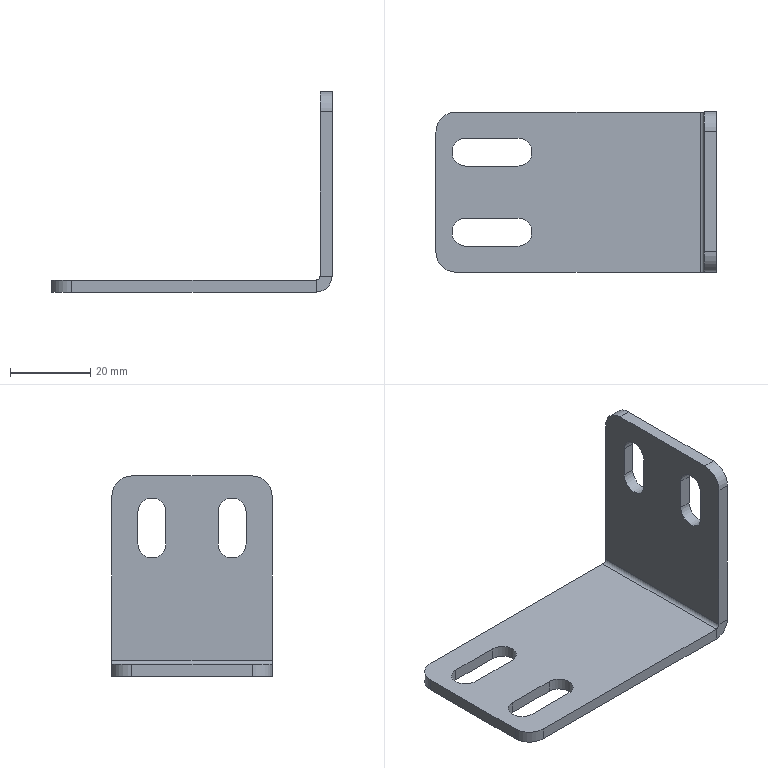Part | STEP file | PN_0072 L-type guardrail connecting plate 70X50_Default<As Machined> | 1 solid | 34 faces | box 70 x 40 x 50 mm | volume 12503 mm3 | plane 20 | cylinder 14 | commonest cylinder face diameters 7 x8 10 x4 2 x1 8 x1